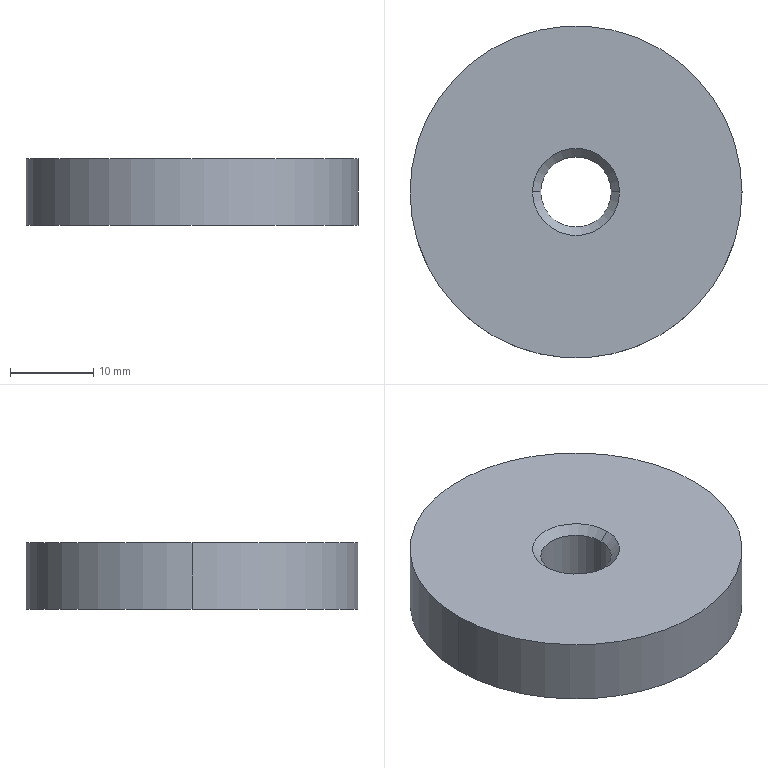Part | STEP file | X77-03030 | 1 solid | 10 faces | box 40 x 40 x 8 mm | volume 9570 mm3 | cone 4 | cylinder 4 | plane 2 | commonest cylinder face diameters 8.5 x2 40 x2
STEP:
#1=CARTESIAN_POINT('',(-1258.703,-4407.704,7.));
#2=VERTEX_POINT('',#1);
#3=CARTESIAN_POINT('',(-1250.203,-4407.704,7.));
#4=VERTEX_POINT('',#3);
#5=CARTESIAN_POINT('',(-1254.453,-4407.704,7.));
#6=DIRECTION('',(0.,0.,1.));
#7=DIRECTION('',(1.,0.,0.));
#8=AXIS2_PLACEMENT_3D('',#5,#6,#7);
#9=CIRCLE('',#8,4.25);
#10=EDGE_CURVE('',#2,#4,#9,.T.);
#11=ORIENTED_EDGE('',*,*,#10,.F.);
#12=CARTESIAN_POINT('',(-1259.703,-4407.704,8.));
#13=VERTEX_POINT('',#12);
#14=CARTESIAN_POINT('',(-1258.703,-4407.704,7.));
#15=DIRECTION('',(-0.7071,0.,0.7071));
#16=VECTOR('',#15,1000.);
#17=LINE('',#14,#16);
#18=EDGE_CURVE('',#2,#13,#17,.T.);
#19=ORIENTED_EDGE('',*,*,#18,.T.);
#20=CARTESIAN_POINT('',(-1249.203,-4407.704,8.));
#21=VERTEX_POINT('',#20);
#22=CARTESIAN_POINT('',(-1254.453,-4407.704,8.));
#23=DIRECTION('',(0.,0.,-1.));
#24=DIRECTION('',(1.,0.,0.));
#25=AXIS2_PLACEMENT_3D('',#22,#23,#24);
#26=CIRCLE('',#25,5.25);
#27=EDGE_CURVE('',#21,#13,#26,.T.);
#28=ORIENTED_EDGE('',*,*,#27,.F.);
#29=CARTESIAN_POINT('',(-1250.203,-4407.704,7.));
#30=DIRECTION('',(0.7071,0.,0.7071));
#31=VECTOR('',#30,1000.);
#32=LINE('',#29,#31);
#33=EDGE_CURVE('',#4,#21,#32,.T.);
#34=ORIENTED_EDGE('',*,*,#33,.F.);
#35=EDGE_LOOP('',(#11,#19,#28,#34));
#36=FACE_OUTER_BOUND('',#35,.T.);
#37=CARTESIAN_POINT('',(-1254.453,-4407.704,7.));
#38=DIRECTION('',(0.,0.,1.));
#39=DIRECTION('',(1.,0.,0.));
#40=AXIS2_PLACEMENT_3D('',#37,#38,#39);
#41=CONICAL_SURFACE('',#40,4.25,0.7854);
#42=ADVANCED_FACE('',(#36),#41,.F.);
#43=CARTESIAN_POINT('',(-1250.203,-4407.704,1.));
#44=VERTEX_POINT('',#43);
#45=CARTESIAN_POINT('',(-1258.703,-4407.704,1.));
#46=VERTEX_POINT('',#45);
#47=CARTESIAN_POINT('',(-1254.453,-4407.704,1.));
#48=DIRECTION('',(0.,0.,-1.));
#49=DIRECTION('',(1.,0.,0.));
#50=AXIS2_PLACEMENT_3D('',#47,#48,#49);
#51=CIRCLE('',#50,4.25);
#52=EDGE_CURVE('',#44,#46,#51,.T.);
#53=ORIENTED_EDGE('',*,*,#52,.F.);
#54=CARTESIAN_POINT('',(-1249.203,-4407.704,0.));
#55=VERTEX_POINT('',#54);
#56=CARTESIAN_POINT('',(-1249.203,-4407.704,0.));
#57=DIRECTION('',(0.7071,0.,-0.7071));
#58=VECTOR('',#57,1000.);
#59=LINE('',#56,#58);
#60=EDGE_CURVE('',#44,#55,#59,.T.);
#61=ORIENTED_EDGE('',*,*,#60,.T.);
#62=CARTESIAN_POINT('',(-1259.703,-4407.704,0.));
#63=VERTEX_POINT('',#62);
#64=CARTESIAN_POINT('',(-1254.453,-4407.704,0.));
#65=DIRECTION('',(0.,0.,1.));
#66=DIRECTION('',(1.,0.,0.));
#67=AXIS2_PLACEMENT_3D('',#64,#65,#66);
#68=CIRCLE('',#67,5.25);
#69=EDGE_CURVE('',#63,#55,#68,.T.);
#70=ORIENTED_EDGE('',*,*,#69,.F.);
#71=CARTESIAN_POINT('',(-1259.703,-4407.704,0.));
#72=DIRECTION('',(-0.7071,0.,-0.7071));
#73=VECTOR('',#72,1000.);
#74=LINE('',#71,#73);
#75=EDGE_CURVE('',#46,#63,#74,.T.);
#76=ORIENTED_EDGE('',*,*,#75,.F.);
#77=EDGE_LOOP('',(#53,#61,#70,#76));
#78=FACE_OUTER_BOUND('',#77,.T.);
#79=CARTESIAN_POINT('',(-1254.453,-4407.704,0.));
#80=DIRECTION('',(0.,0.,-1.));
#81=DIRECTION('',(-1.,0.,0.));
#82=AXIS2_PLACEMENT_3D('',#79,#80,#81);
#83=CONICAL_SURFACE('',#82,5.25,0.7854);
#84=ADVANCED_FACE('',(#78),#83,.F.);
#85=ORIENTED_EDGE('',*,*,#52,.T.);
#86=CARTESIAN_POINT('',(-1258.703,-4407.704,8.));
#87=DIRECTION('',(0.,0.,1.));
#88=VECTOR('',#87,1000.);
#89=LINE('',#86,#88);
#90=EDGE_CURVE('',#46,#2,#89,.T.);
#91=ORIENTED_EDGE('',*,*,#90,.T.);
#92=ORIENTED_EDGE('',*,*,#10,.T.);
#93=CARTESIAN_POINT('',(-1250.203,-4407.704,8.));
#94=DIRECTION('',(0.,0.,1.));
#95=VECTOR('',#94,1000.);
#96=LINE('',#93,#95);
#97=EDGE_CURVE('',#44,#4,#96,.T.);
#98=ORIENTED_EDGE('',*,*,#97,.F.);
#99=EDGE_LOOP('',(#85,#91,#92,#98));
#100=FACE_OUTER_BOUND('',#99,.T.);
#101=CARTESIAN_POINT('',(-1254.453,-4407.704,8.));
#102=DIRECTION('',(0.,0.,1.));
#103=DIRECTION('',(1.,0.,0.));
#104=AXIS2_PLACEMENT_3D('',#101,#102,#103);
#105=CYLINDRICAL_SURFACE('',#104,4.25);
#106=ADVANCED_FACE('',(#100),#105,.F.);
#107=CARTESIAN_POINT('',(-1234.453,-4407.704,8.));
#108=VERTEX_POINT('',#107);
#109=CARTESIAN_POINT('',(-1274.453,-4407.704,8.));
#110=VERTEX_POINT('',#109);
#111=CARTESIAN_POINT('',(-1254.453,-4407.704,8.));
#112=DIRECTION('',(0.,0.,1.));
#113=DIRECTION('',(1.,0.,0.));
#114=AXIS2_PLACEMENT_3D('',#111,#112,#113);
#115=CIRCLE('',#114,20.);
#116=EDGE_CURVE('',#108,#110,#115,.T.);
#117=ORIENTED_EDGE('',*,*,#116,.F.);
#118=CARTESIAN_POINT('',(-1234.453,-4407.704,0.));
#119=VERTEX_POINT('',#118);
#120=CARTESIAN_POINT('',(-1234.453,-4407.704,8.));
#121=DIRECTION('',(0.,0.,-1.));
#122=VECTOR('',#121,1000.);
#123=LINE('',#120,#122);
#124=EDGE_CURVE('',#108,#119,#123,.T.);
#125=ORIENTED_EDGE('',*,*,#124,.T.);
#126=CARTESIAN_POINT('',(-1274.453,-4407.704,0.));
#127=VERTEX_POINT('',#126);
#128=CARTESIAN_POINT('',(-1254.453,-4407.704,0.));
#129=DIRECTION('',(0.,0.,1.));
#130=DIRECTION('',(1.,0.,0.));
#131=AXIS2_PLACEMENT_3D('',#128,#129,#130);
#132=CIRCLE('',#131,20.);
#133=EDGE_CURVE('',#119,#127,#132,.T.);
#134=ORIENTED_EDGE('',*,*,#133,.T.);
#135=CARTESIAN_POINT('',(-1274.453,-4407.704,8.));
#136=DIRECTION('',(0.,0.,-1.));
#137=VECTOR('',#136,1000.);
#138=LINE('',#135,#137);
#139=EDGE_CURVE('',#110,#127,#138,.T.);
#140=ORIENTED_EDGE('',*,*,#139,.F.);
#141=EDGE_LOOP('',(#117,#125,#134,#140));
#142=FACE_OUTER_BOUND('',#141,.T.);
#143=CARTESIAN_POINT('',(-1254.453,-4407.704,8.));
#144=DIRECTION('',(0.,0.,-1.));
#145=DIRECTION('',(-1.,0.,0.));
#146=AXIS2_PLACEMENT_3D('',#143,#144,#145);
#147=CYLINDRICAL_SURFACE('',#146,20.);
#148=ADVANCED_FACE('',(#142),#147,.T.);
#149=ORIENTED_EDGE('',*,*,#124,.F.);
#150=CARTESIAN_POINT('',(-1254.453,-4407.704,8.));
#151=DIRECTION('',(0.,0.,1.));
#152=DIRECTION('',(1.,0.,0.));
#153=AXIS2_PLACEMENT_3D('',#150,#151,#152);
#154=CIRCLE('',#153,20.);
#155=EDGE_CURVE('',#110,#108,#154,.T.);
#156=ORIENTED_EDGE('',*,*,#155,.F.);
#157=ORIENTED_EDGE('',*,*,#139,.T.);
#158=CARTESIAN_POINT('',(-1254.453,-4407.704,0.));
#159=DIRECTION('',(0.,0.,1.));
#160=DIRECTION('',(1.,0.,0.));
#161=AXIS2_PLACEMENT_3D('',#158,#159,#160);
#162=CIRCLE('',#161,20.);
#163=EDGE_CURVE('',#127,#119,#162,.T.);
#164=ORIENTED_EDGE('',*,*,#163,.T.);
#165=EDGE_LOOP('',(#149,#156,#157,#164));
#166=FACE_OUTER_BOUND('',#165,.T.);
#167=CARTESIAN_POINT('',(-1254.453,-4407.704,8.));
#168=DIRECTION('',(0.,0.,-1.));
#169=DIRECTION('',(-1.,0.,0.));
#170=AXIS2_PLACEMENT_3D('',#167,#168,#169);
#171=CYLINDRICAL_SURFACE('',#170,20.);
#172=ADVANCED_FACE('',(#166),#171,.T.);
#173=ORIENTED_EDGE('',*,*,#27,.T.);
#174=CARTESIAN_POINT('',(-1254.453,-4407.704,8.));
#175=DIRECTION('',(0.,0.,-1.));
#176=DIRECTION('',(1.,0.,0.));
#177=AXIS2_PLACEMENT_3D('',#174,#175,#176);
#178=CIRCLE('',#177,5.25);
#179=EDGE_CURVE('',#13,#21,#178,.T.);
#180=ORIENTED_EDGE('',*,*,#179,.T.);
#181=EDGE_LOOP('',(#173,#180));
#182=FACE_BOUND('',#181,.T.);
#183=ORIENTED_EDGE('',*,*,#155,.T.);
#184=ORIENTED_EDGE('',*,*,#116,.T.);
#185=EDGE_LOOP('',(#183,#184));
#186=FACE_OUTER_BOUND('',#185,.T.);
#187=CARTESIAN_POINT('',(-1254.453,-4407.704,8.));
#188=DIRECTION('',(0.,0.,1.));
#189=DIRECTION('',(1.,0.,0.));
#190=AXIS2_PLACEMENT_3D('',#187,#188,#189);
#191=PLANE('',#190);
#192=ADVANCED_FACE('',(#182,#186),#191,.T.);
#193=ORIENTED_EDGE('',*,*,#69,.T.);
#194=CARTESIAN_POINT('',(-1254.453,-4407.704,0.));
#195=DIRECTION('',(0.,0.,1.));
#196=DIRECTION('',(1.,0.,0.));
#197=AXIS2_PLACEMENT_3D('',#194,#195,#196);
#198=CIRCLE('',#197,5.25);
#199=EDGE_CURVE('',#55,#63,#198,.T.);
#200=ORIENTED_EDGE('',*,*,#199,.T.);
#201=EDGE_LOOP('',(#193,#200));
#202=FACE_BOUND('',#201,.T.);
#203=ORIENTED_EDGE('',*,*,#163,.F.);
#204=ORIENTED_EDGE('',*,*,#133,.F.);
#205=EDGE_LOOP('',(#203,#204));
#206=FACE_OUTER_BOUND('',#205,.T.);
#207=CARTESIAN_POINT('',(-1254.453,-4407.704,0.));
#208=DIRECTION('',(0.,0.,1.));
#209=DIRECTION('',(1.,0.,0.));
#210=AXIS2_PLACEMENT_3D('',#207,#208,#209);
#211=PLANE('',#210);
#212=ADVANCED_FACE('',(#202,#206),#211,.F.);
#213=ORIENTED_EDGE('',*,*,#90,.F.);
#214=CARTESIAN_POINT('',(-1254.453,-4407.704,1.));
#215=DIRECTION('',(0.,0.,-1.));
#216=DIRECTION('',(1.,0.,0.));
#217=AXIS2_PLACEMENT_3D('',#214,#215,#216);
#218=CIRCLE('',#217,4.25);
#219=EDGE_CURVE('',#46,#44,#218,.T.);
#220=ORIENTED_EDGE('',*,*,#219,.T.);
#221=ORIENTED_EDGE('',*,*,#97,.T.);
#222=CARTESIAN_POINT('',(-1254.453,-4407.704,7.));
#223=DIRECTION('',(0.,0.,1.));
#224=DIRECTION('',(1.,0.,0.));
#225=AXIS2_PLACEMENT_3D('',#222,#223,#224);
#226=CIRCLE('',#225,4.25);
#227=EDGE_CURVE('',#4,#2,#226,.T.);
#228=ORIENTED_EDGE('',*,*,#227,.T.);
#229=EDGE_LOOP('',(#213,#220,#221,#228));
#230=FACE_OUTER_BOUND('',#229,.T.);
#231=CARTESIAN_POINT('',(-1254.453,-4407.704,8.));
#232=DIRECTION('',(0.,0.,1.));
#233=DIRECTION('',(1.,0.,0.));
#234=AXIS2_PLACEMENT_3D('',#231,#232,#233);
#235=CYLINDRICAL_SURFACE('',#234,4.25);
#236=ADVANCED_FACE('',(#230),#235,.F.);
#237=ORIENTED_EDGE('',*,*,#60,.F.);
#238=ORIENTED_EDGE('',*,*,#219,.F.);
#239=ORIENTED_EDGE('',*,*,#75,.T.);
#240=ORIENTED_EDGE('',*,*,#199,.F.);
#241=EDGE_LOOP('',(#237,#238,#239,#240));
#242=FACE_OUTER_BOUND('',#241,.T.);
#243=CARTESIAN_POINT('',(-1254.453,-4407.704,0.));
#244=DIRECTION('',(0.,0.,-1.));
#245=DIRECTION('',(-1.,0.,0.));
#246=AXIS2_PLACEMENT_3D('',#243,#244,#245);
#247=CONICAL_SURFACE('',#246,5.25,0.7854);
#248=ADVANCED_FACE('',(#242),#247,.F.);
#249=ORIENTED_EDGE('',*,*,#18,.F.);
#250=ORIENTED_EDGE('',*,*,#227,.F.);
#251=ORIENTED_EDGE('',*,*,#33,.T.);
#252=ORIENTED_EDGE('',*,*,#179,.F.);
#253=EDGE_LOOP('',(#249,#250,#251,#252));
#254=FACE_OUTER_BOUND('',#253,.T.);
#255=CARTESIAN_POINT('',(-1254.453,-4407.704,7.));
#256=DIRECTION('',(0.,0.,1.));
#257=DIRECTION('',(1.,0.,0.));
#258=AXIS2_PLACEMENT_3D('',#255,#256,#257);
#259=CONICAL_SURFACE('',#258,4.25,0.7854);
#260=ADVANCED_FACE('',(#254),#259,.F.);
#261=CLOSED_SHELL('',(#42,#84,#106,#148,#172,#192,#212,#236,#248,#260));
#262=MANIFOLD_SOLID_BREP('',#261);
#263=CARTESIAN_POINT('',(0.,0.,0.));
#264=DIRECTION('',(0.,0.,1.));
#265=DIRECTION('',(1.,0.,0.));
#266=AXIS2_PLACEMENT_3D('',#263,#264,#265);
#267=(LENGTH_UNIT()NAMED_UNIT(*)SI_UNIT(.MILLI.,.METRE.));
#268=UNCERTAINTY_MEASURE_WITH_UNIT(LENGTH_MEASURE(0.00001),#267,'','');
#269=(NAMED_UNIT(*)PLANE_ANGLE_UNIT()SI_UNIT($,.RADIAN.));
#270=(NAMED_UNIT(*)SI_UNIT($,.STERADIAN.)SOLID_ANGLE_UNIT());
#271=(GEOMETRIC_REPRESENTATION_CONTEXT(3)GLOBAL_UNCERTAINTY_ASSIGNED_CONTEXT((#268))GLOBAL_UNIT_ASSIGNED_CONTEXT((#267,#269,#270))REPRESENTATION_CONTEXT('',''));
#272=ADVANCED_BREP_SHAPE_REPRESENTATION('',(#262,#266),#271);